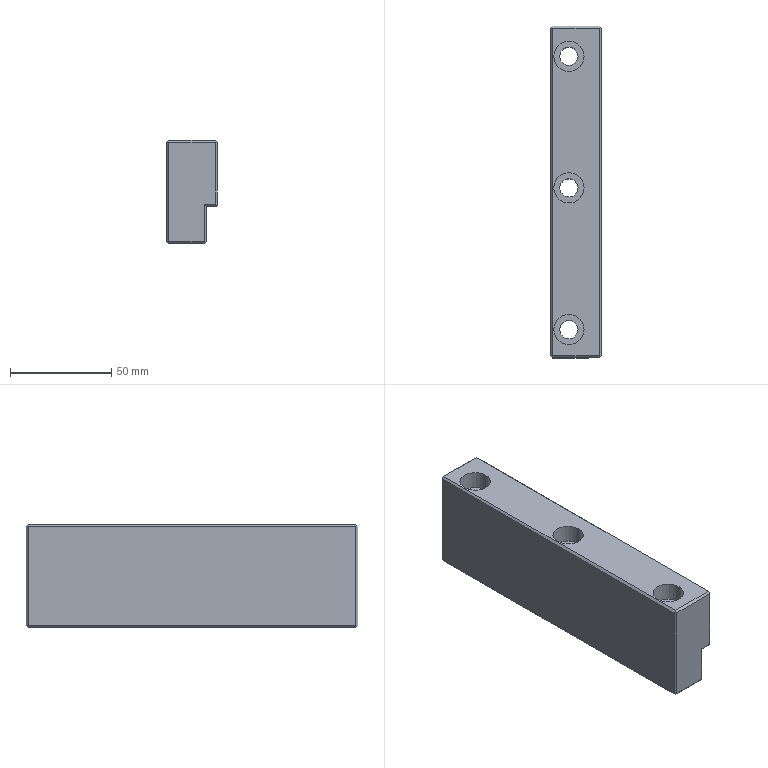Part | Creo | 1 solid | 39 faces | box 25 x 164 x 51 mm | volume 179141 mm3 | plane 27 | cylinder 12 | commonest cylinder face diameters 9 x6 15 x6
STEP:
#1=CARTESIAN_POINT('',(-98.742,211.92,-62.));
#2=VERTEX_POINT('',#1);
#3=CARTESIAN_POINT('',(-98.742,373.92,-62.));
#4=VERTEX_POINT('',#3);
#5=CARTESIAN_POINT('',(-98.742,211.92,-62.));
#6=DIRECTION('',(0.,1.,0.));
#7=VECTOR('',#6,162.);
#8=LINE('',#5,#7);
#9=EDGE_CURVE('',#2,#4,#8,.T.);
#10=ORIENTED_EDGE('',*,*,#9,.T.);
#11=CARTESIAN_POINT('',(-99.242,374.42,-61.5));
#12=VERTEX_POINT('',#11);
#13=CARTESIAN_POINT('',(-98.742,373.92,-62.));
#14=DIRECTION('',(-0.5774,0.5774,0.5774));
#15=VECTOR('',#14,0.866);
#16=LINE('',#13,#15);
#17=EDGE_CURVE('',#4,#12,#16,.T.);
#18=ORIENTED_EDGE('',*,*,#17,.T.);
#19=CARTESIAN_POINT('',(-99.742,373.92,-61.));
#20=VERTEX_POINT('',#19);
#21=CARTESIAN_POINT('',(-99.242,374.42,-61.5));
#22=DIRECTION('',(-0.5774,-0.5774,0.5774));
#23=VECTOR('',#22,0.866);
#24=LINE('',#21,#23);
#25=EDGE_CURVE('',#12,#20,#24,.T.);
#26=ORIENTED_EDGE('',*,*,#25,.T.);
#27=CARTESIAN_POINT('',(-99.742,211.92,-61.));
#28=VERTEX_POINT('',#27);
#29=CARTESIAN_POINT('',(-99.742,211.92,-61.));
#30=DIRECTION('',(0.,1.,0.));
#31=VECTOR('',#30,162.);
#32=LINE('',#29,#31);
#33=EDGE_CURVE('',#28,#20,#32,.T.);
#34=ORIENTED_EDGE('',*,*,#33,.F.);
#35=CARTESIAN_POINT('',(-99.242,211.42,-61.5));
#36=VERTEX_POINT('',#35);
#37=CARTESIAN_POINT('',(-99.742,211.92,-61.));
#38=DIRECTION('',(0.5774,-0.5774,-0.5774));
#39=VECTOR('',#38,0.866);
#40=LINE('',#37,#39);
#41=EDGE_CURVE('',#28,#36,#40,.T.);
#42=ORIENTED_EDGE('',*,*,#41,.T.);
#43=CARTESIAN_POINT('',(-98.742,211.92,-62.));
#44=DIRECTION('',(-0.5774,-0.5774,0.5774));
#45=VECTOR('',#44,0.866);
#46=LINE('',#43,#45);
#47=EDGE_CURVE('',#2,#36,#46,.T.);
#48=ORIENTED_EDGE('',*,*,#47,.F.);
#49=EDGE_LOOP('',(#10,#18,#26,#34,#42,#48));
#50=FACE_OUTER_BOUND('',#49,.F.);
#51=CARTESIAN_POINT('',(-99.242,279.92,-61.5));
#52=DIRECTION('',(-0.7071,0.,-0.7071));
#53=DIRECTION('',(-0.7071,0.,0.7071));
#54=AXIS2_PLACEMENT_3D('',#51,#52,#53);
#55=PLANE('',#54);
#56=ADVANCED_FACE('',(#50),#55,.T.);
#57=CARTESIAN_POINT('',(-81.242,211.92,-62.));
#58=VERTEX_POINT('',#57);
#59=CARTESIAN_POINT('',(-81.242,211.92,-62.));
#60=DIRECTION('',(-1.,0.,0.));
#61=VECTOR('',#60,17.5);
#62=LINE('',#59,#61);
#63=EDGE_CURVE('',#58,#2,#62,.T.);
#64=ORIENTED_EDGE('',*,*,#63,.F.);
#65=CARTESIAN_POINT('',(-81.242,373.92,-62.));
#66=VERTEX_POINT('',#65);
#67=CARTESIAN_POINT('',(-81.242,211.92,-62.));
#68=DIRECTION('',(0.,1.,0.));
#69=VECTOR('',#68,162.);
#70=LINE('',#67,#69);
#71=EDGE_CURVE('',#58,#66,#70,.T.);
#72=ORIENTED_EDGE('',*,*,#71,.T.);
#73=CARTESIAN_POINT('',(-98.742,373.92,-62.));
#74=DIRECTION('',(1.,0.,0.));
#75=VECTOR('',#74,17.5);
#76=LINE('',#73,#75);
#77=EDGE_CURVE('',#4,#66,#76,.T.);
#78=ORIENTED_EDGE('',*,*,#77,.F.);
#79=ORIENTED_EDGE('',*,*,#9,.F.);
#80=EDGE_LOOP('',(#64,#72,#78,#79));
#81=FACE_OUTER_BOUND('',#80,.F.);
#82=CARTESIAN_POINT('',(-86.242,359.92,-62.));
#83=VERTEX_POINT('',#82);
#84=CARTESIAN_POINT('',(-95.242,359.92,-62.));
#85=VERTEX_POINT('',#84);
#86=CARTESIAN_POINT('',(-90.742,359.92,-62.));
#87=DIRECTION('',(0.,0.,1.));
#88=DIRECTION('',(1.,0.,0.));
#89=AXIS2_PLACEMENT_3D('',#86,#87,#88);
#90=CIRCLE('',#89,4.5);
#91=EDGE_CURVE('',#83,#85,#90,.T.);
#92=ORIENTED_EDGE('',*,*,#91,.F.);
#93=CARTESIAN_POINT('',(-90.742,359.92,-62.));
#94=DIRECTION('',(0.,0.,1.));
#95=DIRECTION('',(-1.,0.,0.));
#96=AXIS2_PLACEMENT_3D('',#93,#94,#95);
#97=CIRCLE('',#96,4.5);
#98=EDGE_CURVE('',#85,#83,#97,.T.);
#99=ORIENTED_EDGE('',*,*,#98,.F.);
#100=EDGE_LOOP('',(#92,#99));
#101=FACE_BOUND('',#100,.F.);
#102=CARTESIAN_POINT('',(-86.242,294.92,-62.));
#103=VERTEX_POINT('',#102);
#104=CARTESIAN_POINT('',(-95.242,294.92,-62.));
#105=VERTEX_POINT('',#104);
#106=CARTESIAN_POINT('',(-90.742,294.92,-62.));
#107=DIRECTION('',(0.,0.,1.));
#108=DIRECTION('',(1.,0.,0.));
#109=AXIS2_PLACEMENT_3D('',#106,#107,#108);
#110=CIRCLE('',#109,4.5);
#111=EDGE_CURVE('',#103,#105,#110,.T.);
#112=ORIENTED_EDGE('',*,*,#111,.F.);
#113=CARTESIAN_POINT('',(-90.742,294.92,-62.));
#114=DIRECTION('',(0.,0.,1.));
#115=DIRECTION('',(-1.,0.,0.));
#116=AXIS2_PLACEMENT_3D('',#113,#114,#115);
#117=CIRCLE('',#116,4.5);
#118=EDGE_CURVE('',#105,#103,#117,.T.);
#119=ORIENTED_EDGE('',*,*,#118,.F.);
#120=EDGE_LOOP('',(#112,#119));
#121=FACE_BOUND('',#120,.F.);
#122=CARTESIAN_POINT('',(-86.242,224.92,-62.));
#123=VERTEX_POINT('',#122);
#124=CARTESIAN_POINT('',(-95.242,224.92,-62.));
#125=VERTEX_POINT('',#124);
#126=CARTESIAN_POINT('',(-90.742,224.92,-62.));
#127=DIRECTION('',(0.,0.,1.));
#128=DIRECTION('',(1.,0.,0.));
#129=AXIS2_PLACEMENT_3D('',#126,#127,#128);
#130=CIRCLE('',#129,4.5);
#131=EDGE_CURVE('',#123,#125,#130,.T.);
#132=ORIENTED_EDGE('',*,*,#131,.F.);
#133=CARTESIAN_POINT('',(-90.742,224.92,-62.));
#134=DIRECTION('',(0.,0.,1.));
#135=DIRECTION('',(-1.,0.,0.));
#136=AXIS2_PLACEMENT_3D('',#133,#134,#135);
#137=CIRCLE('',#136,4.5);
#138=EDGE_CURVE('',#125,#123,#137,.T.);
#139=ORIENTED_EDGE('',*,*,#138,.F.);
#140=EDGE_LOOP('',(#132,#139));
#141=FACE_BOUND('',#140,.F.);
#142=CARTESIAN_POINT('',(-80.242,349.92,-62.));
#143=DIRECTION('',(0.,0.,-1.));
#144=DIRECTION('',(1.,0.,0.));
#145=AXIS2_PLACEMENT_3D('',#142,#143,#144);
#146=PLANE('',#145);
#147=ADVANCED_FACE('',(#81,#101,#121,#141),#146,.T.);
#148=ORIENTED_EDGE('',*,*,#63,.T.);
#149=ORIENTED_EDGE('',*,*,#47,.T.);
#150=CARTESIAN_POINT('',(-98.742,210.92,-61.));
#151=VERTEX_POINT('',#150);
#152=CARTESIAN_POINT('',(-99.242,211.42,-61.5));
#153=DIRECTION('',(0.5774,-0.5774,0.5774));
#154=VECTOR('',#153,0.866);
#155=LINE('',#152,#154);
#156=EDGE_CURVE('',#36,#151,#155,.T.);
#157=ORIENTED_EDGE('',*,*,#156,.T.);
#158=CARTESIAN_POINT('',(-81.242,210.92,-61.));
#159=VERTEX_POINT('',#158);
#160=CARTESIAN_POINT('',(-81.242,210.92,-61.));
#161=DIRECTION('',(-1.,0.,0.));
#162=VECTOR('',#161,17.5);
#163=LINE('',#160,#162);
#164=EDGE_CURVE('',#159,#151,#163,.T.);
#165=ORIENTED_EDGE('',*,*,#164,.F.);
#166=CARTESIAN_POINT('',(-80.742,211.42,-61.5));
#167=VERTEX_POINT('',#166);
#168=CARTESIAN_POINT('',(-81.242,210.92,-61.));
#169=DIRECTION('',(0.5774,0.5774,-0.5774));
#170=VECTOR('',#169,0.866);
#171=LINE('',#168,#170);
#172=EDGE_CURVE('',#159,#167,#171,.T.);
#173=ORIENTED_EDGE('',*,*,#172,.T.);
#174=CARTESIAN_POINT('',(-80.742,211.42,-61.5));
#175=DIRECTION('',(-0.5774,0.5774,-0.5774));
#176=VECTOR('',#175,0.866);
#177=LINE('',#174,#176);
#178=EDGE_CURVE('',#167,#58,#177,.T.);
#179=ORIENTED_EDGE('',*,*,#178,.T.);
#180=EDGE_LOOP('',(#148,#149,#157,#165,#173,#179));
#181=FACE_OUTER_BOUND('',#180,.F.);
#182=CARTESIAN_POINT('',(-89.992,211.42,-61.5));
#183=DIRECTION('',(0.,-0.7071,-0.7071));
#184=DIRECTION('',(0.,-0.7071,0.7071));
#185=AXIS2_PLACEMENT_3D('',#182,#183,#184);
#186=PLANE('',#185);
#187=ADVANCED_FACE('',(#181),#186,.T.);
#188=CARTESIAN_POINT('',(-98.742,210.92,-12.));
#189=VERTEX_POINT('',#188);
#190=CARTESIAN_POINT('',(-98.742,210.92,-61.));
#191=DIRECTION('',(0.,0.,1.));
#192=VECTOR('',#191,49.);
#193=LINE('',#190,#192);
#194=EDGE_CURVE('',#151,#189,#193,.T.);
#195=ORIENTED_EDGE('',*,*,#194,.F.);
#196=ORIENTED_EDGE('',*,*,#156,.F.);
#197=ORIENTED_EDGE('',*,*,#41,.F.);
#198=CARTESIAN_POINT('',(-99.742,211.92,-12.));
#199=VERTEX_POINT('',#198);
#200=CARTESIAN_POINT('',(-99.742,211.92,-61.));
#201=DIRECTION('',(0.,0.,1.));
#202=VECTOR('',#201,49.);
#203=LINE('',#200,#202);
#204=EDGE_CURVE('',#28,#199,#203,.T.);
#205=ORIENTED_EDGE('',*,*,#204,.T.);
#206=CARTESIAN_POINT('',(-99.242,211.42,-11.5));
#207=VERTEX_POINT('',#206);
#208=CARTESIAN_POINT('',(-99.242,211.42,-11.5));
#209=DIRECTION('',(-0.5774,0.5774,-0.5774));
#210=VECTOR('',#209,0.866);
#211=LINE('',#208,#210);
#212=EDGE_CURVE('',#207,#199,#211,.T.);
#213=ORIENTED_EDGE('',*,*,#212,.F.);
#214=CARTESIAN_POINT('',(-99.242,211.42,-11.5));
#215=DIRECTION('',(0.5774,-0.5774,-0.5774));
#216=VECTOR('',#215,0.866);
#217=LINE('',#214,#216);
#218=EDGE_CURVE('',#207,#189,#217,.T.);
#219=ORIENTED_EDGE('',*,*,#218,.T.);
#220=EDGE_LOOP('',(#195,#196,#197,#205,#213,#219));
#221=FACE_OUTER_BOUND('',#220,.F.);
#222=CARTESIAN_POINT('',(-99.242,211.42,-29.));
#223=DIRECTION('',(-0.7071,-0.7071,0.));
#224=DIRECTION('',(0.7071,-0.7071,0.));
#225=AXIS2_PLACEMENT_3D('',#222,#223,#224);
#226=PLANE('',#225);
#227=ADVANCED_FACE('',(#221),#226,.T.);
#228=CARTESIAN_POINT('',(-81.242,210.92,-42.5));
#229=VERTEX_POINT('',#228);
#230=CARTESIAN_POINT('',(-81.242,210.92,-42.5));
#231=DIRECTION('',(0.,0.,-1.));
#232=VECTOR('',#231,18.5);
#233=LINE('',#230,#232);
#234=EDGE_CURVE('',#229,#159,#233,.T.);
#235=ORIENTED_EDGE('',*,*,#234,.T.);
#236=ORIENTED_EDGE('',*,*,#164,.T.);
#237=ORIENTED_EDGE('',*,*,#194,.T.);
#238=CARTESIAN_POINT('',(-75.742,210.92,-12.));
#239=VERTEX_POINT('',#238);
#240=CARTESIAN_POINT('',(-98.742,210.92,-12.));
#241=DIRECTION('',(1.,0.,0.));
#242=VECTOR('',#241,23.);
#243=LINE('',#240,#242);
#244=EDGE_CURVE('',#189,#239,#243,.T.);
#245=ORIENTED_EDGE('',*,*,#244,.T.);
#246=CARTESIAN_POINT('',(-75.742,210.92,-42.5));
#247=VERTEX_POINT('',#246);
#248=CARTESIAN_POINT('',(-75.742,210.92,-12.));
#249=DIRECTION('',(0.,0.,-1.));
#250=VECTOR('',#249,30.5);
#251=LINE('',#248,#250);
#252=EDGE_CURVE('',#239,#247,#251,.T.);
#253=ORIENTED_EDGE('',*,*,#252,.T.);
#254=CARTESIAN_POINT('',(-75.742,210.92,-42.5));
#255=DIRECTION('',(-1.,0.,0.));
#256=VECTOR('',#255,5.5);
#257=LINE('',#254,#256);
#258=EDGE_CURVE('',#247,#229,#257,.T.);
#259=ORIENTED_EDGE('',*,*,#258,.T.);
#260=EDGE_LOOP('',(#235,#236,#237,#245,#253,#259));
#261=FACE_OUTER_BOUND('',#260,.F.);
#262=CARTESIAN_POINT('',(-80.242,210.92,-41.));
#263=DIRECTION('',(0.,-1.,0.));
#264=DIRECTION('',(0.,0.,-1.));
#265=AXIS2_PLACEMENT_3D('',#262,#263,#264);
#266=PLANE('',#265);
#267=ADVANCED_FACE('',(#261),#266,.T.);
#268=ORIENTED_EDGE('',*,*,#172,.F.);
#269=ORIENTED_EDGE('',*,*,#234,.F.);
#270=CARTESIAN_POINT('',(-80.242,211.92,-43.5));
#271=VERTEX_POINT('',#270);
#272=CARTESIAN_POINT('',(-80.242,211.92,-43.5));
#273=DIRECTION('',(-0.5774,-0.5774,0.5774));
#274=VECTOR('',#273,1.732);
#275=LINE('',#272,#274);
#276=EDGE_CURVE('',#271,#229,#275,.T.);
#277=ORIENTED_EDGE('',*,*,#276,.F.);
#278=CARTESIAN_POINT('',(-80.242,211.92,-61.));
#279=VERTEX_POINT('',#278);
#280=CARTESIAN_POINT('',(-80.242,211.92,-61.));
#281=DIRECTION('',(0.,0.,1.));
#282=VECTOR('',#281,17.5);
#283=LINE('',#280,#282);
#284=EDGE_CURVE('',#279,#271,#283,.T.);
#285=ORIENTED_EDGE('',*,*,#284,.F.);
#286=CARTESIAN_POINT('',(-80.242,211.92,-61.));
#287=DIRECTION('',(-0.5774,-0.5774,-0.5774));
#288=VECTOR('',#287,0.866);
#289=LINE('',#286,#288);
#290=EDGE_CURVE('',#279,#167,#289,.T.);
#291=ORIENTED_EDGE('',*,*,#290,.T.);
#292=EDGE_LOOP('',(#268,#269,#277,#285,#291));
#293=FACE_OUTER_BOUND('',#292,.F.);
#294=CARTESIAN_POINT('',(-80.742,211.42,-51.5));
#295=DIRECTION('',(0.7071,-0.7071,0.));
#296=DIRECTION('',(-0.7071,-0.7071,0.));
#297=AXIS2_PLACEMENT_3D('',#294,#295,#296);
#298=PLANE('',#297);
#299=ADVANCED_FACE('',(#293),#298,.T.);
#300=CARTESIAN_POINT('',(-75.242,211.92,-43.5));
#301=VERTEX_POINT('',#300);
#302=CARTESIAN_POINT('',(-75.242,211.92,-43.5));
#303=DIRECTION('',(-1.,0.,0.));
#304=VECTOR('',#303,5.);
#305=LINE('',#302,#304);
#306=EDGE_CURVE('',#301,#271,#305,.T.);
#307=ORIENTED_EDGE('',*,*,#306,.T.);
#308=ORIENTED_EDGE('',*,*,#276,.T.);
#309=ORIENTED_EDGE('',*,*,#258,.F.);
#310=CARTESIAN_POINT('',(-74.992,211.67,-43.25));
#311=VERTEX_POINT('',#310);
#312=CARTESIAN_POINT('',(-75.742,210.92,-42.5));
#313=DIRECTION('',(0.5774,0.5774,-0.5774));
#314=VECTOR('',#313,1.299);
#315=LINE('',#312,#314);
#316=EDGE_CURVE('',#247,#311,#315,.T.);
#317=ORIENTED_EDGE('',*,*,#316,.T.);
#318=CARTESIAN_POINT('',(-74.992,211.67,-43.25));
#319=DIRECTION('',(-0.5774,0.5774,-0.5774));
#320=VECTOR('',#319,0.433);
#321=LINE('',#318,#320);
#322=EDGE_CURVE('',#311,#301,#321,.T.);
#323=ORIENTED_EDGE('',*,*,#322,.T.);
#324=EDGE_LOOP('',(#307,#308,#309,#317,#323));
#325=FACE_OUTER_BOUND('',#324,.F.);
#326=CARTESIAN_POINT('',(-77.492,211.42,-43.));
#327=DIRECTION('',(0.,-0.7071,-0.7071));
#328=DIRECTION('',(0.,-0.7071,0.7071));
#329=AXIS2_PLACEMENT_3D('',#326,#327,#328);
#330=PLANE('',#329);
#331=ADVANCED_FACE('',(#325),#330,.T.);
#332=CARTESIAN_POINT('',(-80.242,373.92,-43.5));
#333=VERTEX_POINT('',#332);
#334=CARTESIAN_POINT('',(-75.242,373.92,-43.5));
#335=VERTEX_POINT('',#334);
#336=CARTESIAN_POINT('',(-80.242,373.92,-43.5));
#337=DIRECTION('',(1.,0.,0.));
#338=VECTOR('',#337,5.);
#339=LINE('',#336,#338);
#340=EDGE_CURVE('',#333,#335,#339,.T.);
#341=ORIENTED_EDGE('',*,*,#340,.F.);
#342=CARTESIAN_POINT('',(-80.242,373.92,-43.5));
#343=DIRECTION('',(0.,-1.,0.));
#344=VECTOR('',#343,162.);
#345=LINE('',#342,#344);
#346=EDGE_CURVE('',#333,#271,#345,.T.);
#347=ORIENTED_EDGE('',*,*,#346,.T.);
#348=ORIENTED_EDGE('',*,*,#306,.F.);
#349=CARTESIAN_POINT('',(-75.242,211.92,-43.5));
#350=DIRECTION('',(0.,1.,0.));
#351=VECTOR('',#350,162.);
#352=LINE('',#349,#351);
#353=EDGE_CURVE('',#301,#335,#352,.T.);
#354=ORIENTED_EDGE('',*,*,#353,.T.);
#355=EDGE_LOOP('',(#341,#347,#348,#354));
#356=FACE_OUTER_BOUND('',#355,.F.);
#357=CARTESIAN_POINT('',(-74.742,349.92,-43.5));
#358=DIRECTION('',(0.,0.,-1.));
#359=DIRECTION('',(1.,0.,0.));
#360=AXIS2_PLACEMENT_3D('',#357,#358,#359);
#361=PLANE('',#360);
#362=ADVANCED_FACE('',(#356),#361,.T.);
#363=CARTESIAN_POINT('',(-74.992,374.17,-43.25));
#364=VERTEX_POINT('',#363);
#365=CARTESIAN_POINT('',(-75.742,374.92,-42.5));
#366=VERTEX_POINT('',#365);
#367=CARTESIAN_POINT('',(-74.992,374.17,-43.25));
#368=DIRECTION('',(-0.5774,0.5774,0.5774));
#369=VECTOR('',#368,1.299);
#370=LINE('',#367,#369);
#371=EDGE_CURVE('',#364,#366,#370,.T.);
#372=ORIENTED_EDGE('',*,*,#371,.T.);
#373=CARTESIAN_POINT('',(-80.242,374.92,-42.5));
#374=VERTEX_POINT('',#373);
#375=CARTESIAN_POINT('',(-80.242,374.92,-42.5));
#376=DIRECTION('',(1.,0.,0.));
#377=VECTOR('',#376,4.5);
#378=LINE('',#375,#377);
#379=EDGE_CURVE('',#374,#366,#378,.T.);
#380=ORIENTED_EDGE('',*,*,#379,.F.);
#381=CARTESIAN_POINT('',(-80.242,374.92,-42.5));
#382=DIRECTION('',(0.,-0.7071,-0.7071));
#383=VECTOR('',#382,1.414);
#384=LINE('',#381,#383);
#385=EDGE_CURVE('',#374,#333,#384,.T.);
#386=ORIENTED_EDGE('',*,*,#385,.T.);
#387=ORIENTED_EDGE('',*,*,#340,.T.);
#388=CARTESIAN_POINT('',(-75.242,373.92,-43.5));
#389=DIRECTION('',(0.5774,0.5774,0.5774));
#390=VECTOR('',#389,0.433);
#391=LINE('',#388,#390);
#392=EDGE_CURVE('',#335,#364,#391,.T.);
#393=ORIENTED_EDGE('',*,*,#392,.T.);
#394=EDGE_LOOP('',(#372,#380,#386,#387,#393));
#395=FACE_OUTER_BOUND('',#394,.F.);
#396=CARTESIAN_POINT('',(-77.492,374.42,-43.));
#397=DIRECTION('',(0.,0.7071,-0.7071));
#398=DIRECTION('',(0.,0.7071,0.7071));
#399=AXIS2_PLACEMENT_3D('',#396,#397,#398);
#400=PLANE('',#399);
#401=ADVANCED_FACE('',(#395),#400,.T.);
#402=CARTESIAN_POINT('',(-74.742,373.92,-43.));
#403=VERTEX_POINT('',#402);
#404=CARTESIAN_POINT('',(-74.742,373.92,-12.));
#405=VERTEX_POINT('',#404);
#406=CARTESIAN_POINT('',(-74.742,373.92,-43.));
#407=DIRECTION('',(0.,0.,1.));
#408=VECTOR('',#407,31.);
#409=LINE('',#406,#408);
#410=EDGE_CURVE('',#403,#405,#409,.T.);
#411=ORIENTED_EDGE('',*,*,#410,.T.);
#412=CARTESIAN_POINT('',(-75.242,374.42,-11.5));
#413=VERTEX_POINT('',#412);
#414=CARTESIAN_POINT('',(-74.742,373.92,-12.));
#415=DIRECTION('',(-0.5774,0.5774,0.5774));
#416=VECTOR('',#415,0.866);
#417=LINE('',#414,#416);
#418=EDGE_CURVE('',#405,#413,#417,.T.);
#419=ORIENTED_EDGE('',*,*,#418,.T.);
#420=CARTESIAN_POINT('',(-75.742,374.92,-12.));
#421=VERTEX_POINT('',#420);
#422=CARTESIAN_POINT('',(-75.242,374.42,-11.5));
#423=DIRECTION('',(-0.5774,0.5774,-0.5774));
#424=VECTOR('',#423,0.866);
#425=LINE('',#422,#424);
#426=EDGE_CURVE('',#413,#421,#425,.T.);
#427=ORIENTED_EDGE('',*,*,#426,.T.);
#428=CARTESIAN_POINT('',(-75.742,374.92,-42.5));
#429=DIRECTION('',(0.,0.,1.));
#430=VECTOR('',#429,30.5);
#431=LINE('',#428,#430);
#432=EDGE_CURVE('',#366,#421,#431,.T.);
#433=ORIENTED_EDGE('',*,*,#432,.F.);
#434=ORIENTED_EDGE('',*,*,#371,.F.);
#435=CARTESIAN_POINT('',(-74.992,374.17,-43.25));
#436=DIRECTION('',(0.5774,-0.5774,0.5774));
#437=VECTOR('',#436,0.433);
#438=LINE('',#435,#437);
#439=EDGE_CURVE('',#364,#403,#438,.T.);
#440=ORIENTED_EDGE('',*,*,#439,.T.);
#441=EDGE_LOOP('',(#411,#419,#427,#433,#434,#440));
#442=FACE_OUTER_BOUND('',#441,.F.);
#443=CARTESIAN_POINT('',(-75.242,374.42,-21.));
#444=DIRECTION('',(0.7071,0.7071,0.));
#445=DIRECTION('',(-0.7071,0.7071,0.));
#446=AXIS2_PLACEMENT_3D('',#443,#444,#445);
#447=PLANE('',#446);
#448=ADVANCED_FACE('',(#442),#447,.T.);
#449=CARTESIAN_POINT('',(-74.742,211.92,-12.));
#450=VERTEX_POINT('',#449);
#451=CARTESIAN_POINT('',(-74.742,211.92,-43.));
#452=VERTEX_POINT('',#451);
#453=CARTESIAN_POINT('',(-74.742,211.92,-12.));
#454=DIRECTION('',(0.,0.,-1.));
#455=VECTOR('',#454,31.);
#456=LINE('',#453,#455);
#457=EDGE_CURVE('',#450,#452,#456,.T.);
#458=ORIENTED_EDGE('',*,*,#457,.F.);
#459=CARTESIAN_POINT('',(-74.742,211.92,-12.));
#460=DIRECTION('',(0.,1.,0.));
#461=VECTOR('',#460,162.);
#462=LINE('',#459,#461);
#463=EDGE_CURVE('',#450,#405,#462,.T.);
#464=ORIENTED_EDGE('',*,*,#463,.T.);
#465=ORIENTED_EDGE('',*,*,#410,.F.);
#466=CARTESIAN_POINT('',(-74.742,211.92,-43.));
#467=DIRECTION('',(0.,1.,0.));
#468=VECTOR('',#467,162.);
#469=LINE('',#466,#468);
#470=EDGE_CURVE('',#452,#403,#469,.T.);
#471=ORIENTED_EDGE('',*,*,#470,.F.);
#472=EDGE_LOOP('',(#458,#464,#465,#471));
#473=FACE_OUTER_BOUND('',#472,.F.);
#474=CARTESIAN_POINT('',(-74.742,349.92,-1.));
#475=DIRECTION('',(1.,0.,0.));
#476=DIRECTION('',(0.,0.,1.));
#477=AXIS2_PLACEMENT_3D('',#474,#475,#476);
#478=PLANE('',#477);
#479=ADVANCED_FACE('',(#473),#478,.T.);
#480=CARTESIAN_POINT('',(-75.242,211.42,-11.5));
#481=VERTEX_POINT('',#480);
#482=CARTESIAN_POINT('',(-74.742,211.92,-12.));
#483=DIRECTION('',(-0.5774,-0.5774,0.5774));
#484=VECTOR('',#483,0.866);
#485=LINE('',#482,#484);
#486=EDGE_CURVE('',#450,#481,#485,.T.);
#487=ORIENTED_EDGE('',*,*,#486,.F.);
#488=ORIENTED_EDGE('',*,*,#457,.T.);
#489=CARTESIAN_POINT('',(-74.742,211.92,-43.));
#490=DIRECTION('',(-0.5774,-0.5774,-0.5774));
#491=VECTOR('',#490,0.433);
#492=LINE('',#489,#491);
#493=EDGE_CURVE('',#452,#311,#492,.T.);
#494=ORIENTED_EDGE('',*,*,#493,.T.);
#495=ORIENTED_EDGE('',*,*,#316,.F.);
#496=ORIENTED_EDGE('',*,*,#252,.F.);
#497=CARTESIAN_POINT('',(-75.742,210.92,-12.));
#498=DIRECTION('',(0.5774,0.5774,0.5774));
#499=VECTOR('',#498,0.866);
#500=LINE('',#497,#499);
#501=EDGE_CURVE('',#239,#481,#500,.T.);
#502=ORIENTED_EDGE('',*,*,#501,.T.);
#503=EDGE_LOOP('',(#487,#488,#494,#495,#496,#502));
#504=FACE_OUTER_BOUND('',#503,.F.);
#505=CARTESIAN_POINT('',(-75.242,211.42,-21.));
#506=DIRECTION('',(0.7071,-0.7071,0.));
#507=DIRECTION('',(-0.7071,-0.7071,0.));
#508=AXIS2_PLACEMENT_3D('',#505,#506,#507);
#509=PLANE('',#508);
#510=ADVANCED_FACE('',(#504),#509,.T.);
#511=CARTESIAN_POINT('',(-75.742,211.92,-11.));
#512=VERTEX_POINT('',#511);
#513=CARTESIAN_POINT('',(-75.742,373.92,-11.));
#514=VERTEX_POINT('',#513);
#515=CARTESIAN_POINT('',(-75.742,211.92,-11.));
#516=DIRECTION('',(0.,1.,0.));
#517=VECTOR('',#516,162.);
#518=LINE('',#515,#517);
#519=EDGE_CURVE('',#512,#514,#518,.T.);
#520=ORIENTED_EDGE('',*,*,#519,.T.);
#521=CARTESIAN_POINT('',(-75.742,373.92,-11.));
#522=DIRECTION('',(0.5774,0.5774,-0.5774));
#523=VECTOR('',#522,0.866);
#524=LINE('',#521,#523);
#525=EDGE_CURVE('',#514,#413,#524,.T.);
#526=ORIENTED_EDGE('',*,*,#525,.T.);
#527=ORIENTED_EDGE('',*,*,#418,.F.);
#528=ORIENTED_EDGE('',*,*,#463,.F.);
#529=ORIENTED_EDGE('',*,*,#486,.T.);
#530=CARTESIAN_POINT('',(-75.242,211.42,-11.5));
#531=DIRECTION('',(-0.5774,0.5774,0.5774));
#532=VECTOR('',#531,0.866);
#533=LINE('',#530,#532);
#534=EDGE_CURVE('',#481,#512,#533,.T.);
#535=ORIENTED_EDGE('',*,*,#534,.T.);
#536=EDGE_LOOP('',(#520,#526,#527,#528,#529,#535));
#537=FACE_OUTER_BOUND('',#536,.F.);
#538=CARTESIAN_POINT('',(-75.242,279.92,-11.5));
#539=DIRECTION('',(0.7071,0.,0.7071));
#540=DIRECTION('',(0.7071,0.,-0.7071));
#541=AXIS2_PLACEMENT_3D('',#538,#539,#540);
#542=PLANE('',#541);
#543=ADVANCED_FACE('',(#537),#542,.T.);
#544=CARTESIAN_POINT('',(-98.742,211.92,-11.));
#545=VERTEX_POINT('',#544);
#546=CARTESIAN_POINT('',(-98.742,373.92,-11.));
#547=VERTEX_POINT('',#546);
#548=CARTESIAN_POINT('',(-98.742,211.92,-11.));
#549=DIRECTION('',(0.,1.,0.));
#550=VECTOR('',#549,162.);
#551=LINE('',#548,#550);
#552=EDGE_CURVE('',#545,#547,#551,.T.);
#553=ORIENTED_EDGE('',*,*,#552,.T.);
#554=CARTESIAN_POINT('',(-75.742,373.92,-11.));
#555=DIRECTION('',(-1.,0.,0.));
#556=VECTOR('',#555,23.);
#557=LINE('',#554,#556);
#558=EDGE_CURVE('',#514,#547,#557,.T.);
#559=ORIENTED_EDGE('',*,*,#558,.F.);
#560=ORIENTED_EDGE('',*,*,#519,.F.);
#561=CARTESIAN_POINT('',(-98.742,211.92,-11.));
#562=DIRECTION('',(1.,0.,0.));
#563=VECTOR('',#562,23.);
#564=LINE('',#561,#563);
#565=EDGE_CURVE('',#545,#512,#564,.T.);
#566=ORIENTED_EDGE('',*,*,#565,.F.);
#567=EDGE_LOOP('',(#553,#559,#560,#566));
#568=FACE_OUTER_BOUND('',#567,.F.);
#569=CARTESIAN_POINT('',(-83.242,294.92,-11.));
#570=VERTEX_POINT('',#569);
#571=CARTESIAN_POINT('',(-98.242,294.92,-11.));
#572=VERTEX_POINT('',#571);
#573=CARTESIAN_POINT('',(-90.742,294.92,-11.));
#574=DIRECTION('',(0.,0.,-1.));
#575=DIRECTION('',(1.,0.,0.));
#576=AXIS2_PLACEMENT_3D('',#573,#574,#575);
#577=CIRCLE('',#576,7.5);
#578=EDGE_CURVE('',#570,#572,#577,.T.);
#579=ORIENTED_EDGE('',*,*,#578,.F.);
#580=CARTESIAN_POINT('',(-90.742,294.92,-11.));
#581=DIRECTION('',(0.,0.,-1.));
#582=DIRECTION('',(-1.,0.,0.));
#583=AXIS2_PLACEMENT_3D('',#580,#581,#582);
#584=CIRCLE('',#583,7.5);
#585=EDGE_CURVE('',#572,#570,#584,.T.);
#586=ORIENTED_EDGE('',*,*,#585,.F.);
#587=EDGE_LOOP('',(#579,#586));
#588=FACE_BOUND('',#587,.F.);
#589=CARTESIAN_POINT('',(-83.242,359.92,-11.));
#590=VERTEX_POINT('',#589);
#591=CARTESIAN_POINT('',(-98.242,359.92,-11.));
#592=VERTEX_POINT('',#591);
#593=CARTESIAN_POINT('',(-90.742,359.92,-11.));
#594=DIRECTION('',(0.,0.,-1.));
#595=DIRECTION('',(1.,0.,0.));
#596=AXIS2_PLACEMENT_3D('',#593,#594,#595);
#597=CIRCLE('',#596,7.5);
#598=EDGE_CURVE('',#590,#592,#597,.T.);
#599=ORIENTED_EDGE('',*,*,#598,.F.);
#600=CARTESIAN_POINT('',(-90.742,359.92,-11.));
#601=DIRECTION('',(0.,0.,-1.));
#602=DIRECTION('',(-1.,0.,0.));
#603=AXIS2_PLACEMENT_3D('',#600,#601,#602);
#604=CIRCLE('',#603,7.5);
#605=EDGE_CURVE('',#592,#590,#604,.T.);
#606=ORIENTED_EDGE('',*,*,#605,.F.);
#607=EDGE_LOOP('',(#599,#606));
#608=FACE_BOUND('',#607,.F.);
#609=CARTESIAN_POINT('',(-83.242,224.92,-11.));
#610=VERTEX_POINT('',#609);
#611=CARTESIAN_POINT('',(-98.242,224.92,-11.));
#612=VERTEX_POINT('',#611);
#613=CARTESIAN_POINT('',(-90.742,224.92,-11.));
#614=DIRECTION('',(0.,0.,-1.));
#615=DIRECTION('',(1.,0.,0.));
#616=AXIS2_PLACEMENT_3D('',#613,#614,#615);
#617=CIRCLE('',#616,7.5);
#618=EDGE_CURVE('',#610,#612,#617,.T.);
#619=ORIENTED_EDGE('',*,*,#618,.F.);
#620=CARTESIAN_POINT('',(-90.742,224.92,-11.));
#621=DIRECTION('',(0.,0.,-1.));
#622=DIRECTION('',(-1.,0.,0.));
#623=AXIS2_PLACEMENT_3D('',#620,#621,#622);
#624=CIRCLE('',#623,7.5);
#625=EDGE_CURVE('',#612,#610,#624,.T.);
#626=ORIENTED_EDGE('',*,*,#625,.F.);
#627=EDGE_LOOP('',(#619,#626));
#628=FACE_BOUND('',#627,.F.);
#629=CARTESIAN_POINT('',(-99.742,349.92,-11.));
#630=DIRECTION('',(0.,0.,1.));
#631=DIRECTION('',(-1.,0.,0.));
#632=AXIS2_PLACEMENT_3D('',#629,#630,#631);
#633=PLANE('',#632);
#634=ADVANCED_FACE('',(#568,#588,#608,#628),#633,.T.);
#635=CARTESIAN_POINT('',(-98.742,211.92,-11.));
#636=DIRECTION('',(-0.5774,-0.5774,-0.5774));
#637=VECTOR('',#636,0.866);
#638=LINE('',#635,#637);
#639=EDGE_CURVE('',#545,#207,#638,.T.);
#640=ORIENTED_EDGE('',*,*,#639,.T.);
#641=ORIENTED_EDGE('',*,*,#212,.T.);
#642=CARTESIAN_POINT('',(-99.742,373.92,-12.));
#643=VERTEX_POINT('',#642);
#644=CARTESIAN_POINT('',(-99.742,211.92,-12.));
#645=DIRECTION('',(0.,1.,0.));
#646=VECTOR('',#645,162.);
#647=LINE('',#644,#646);
#648=EDGE_CURVE('',#199,#643,#647,.T.);
#649=ORIENTED_EDGE('',*,*,#648,.T.);
#650=CARTESIAN_POINT('',(-99.242,374.42,-11.5));
#651=VERTEX_POINT('',#650);
#652=CARTESIAN_POINT('',(-99.742,373.92,-12.));
#653=DIRECTION('',(0.5774,0.5774,0.5774));
#654=VECTOR('',#653,0.866);
#655=LINE('',#652,#654);
#656=EDGE_CURVE('',#643,#651,#655,.T.);
#657=ORIENTED_EDGE('',*,*,#656,.T.);
#658=CARTESIAN_POINT('',(-98.742,373.92,-11.));
#659=DIRECTION('',(-0.5774,0.5774,-0.5774));
#660=VECTOR('',#659,0.866);
#661=LINE('',#658,#660);
#662=EDGE_CURVE('',#547,#651,#661,.T.);
#663=ORIENTED_EDGE('',*,*,#662,.F.);
#664=ORIENTED_EDGE('',*,*,#552,.F.);
#665=EDGE_LOOP('',(#640,#641,#649,#657,#663,#664));
#666=FACE_OUTER_BOUND('',#665,.F.);
#667=CARTESIAN_POINT('',(-99.242,279.92,-11.5));
#668=DIRECTION('',(-0.7071,0.,0.7071));
#669=DIRECTION('',(0.7071,0.,0.7071));
#670=AXIS2_PLACEMENT_3D('',#667,#668,#669);
#671=PLANE('',#670);
#672=ADVANCED_FACE('',(#666),#671,.T.);
#673=ORIENTED_EDGE('',*,*,#244,.F.);
#674=ORIENTED_EDGE('',*,*,#218,.F.);
#675=ORIENTED_EDGE('',*,*,#639,.F.);
#676=ORIENTED_EDGE('',*,*,#565,.T.);
#677=ORIENTED_EDGE('',*,*,#534,.F.);
#678=ORIENTED_EDGE('',*,*,#501,.F.);
#679=EDGE_LOOP('',(#673,#674,#675,#676,#677,#678));
#680=FACE_OUTER_BOUND('',#679,.F.);
#681=CARTESIAN_POINT('',(-87.242,211.42,-11.5));
#682=DIRECTION('',(0.,-0.7071,0.7071));
#683=DIRECTION('',(0.,-0.7071,-0.7071));
#684=AXIS2_PLACEMENT_3D('',#681,#682,#683);
#685=PLANE('',#684);
#686=ADVANCED_FACE('',(#680),#685,.T.);
#687=ORIENTED_EDGE('',*,*,#204,.F.);
#688=ORIENTED_EDGE('',*,*,#33,.T.);
#689=CARTESIAN_POINT('',(-99.742,373.92,-12.));
#690=DIRECTION('',(0.,0.,-1.));
#691=VECTOR('',#690,49.);
#692=LINE('',#689,#691);
#693=EDGE_CURVE('',#643,#20,#692,.T.);
#694=ORIENTED_EDGE('',*,*,#693,.F.);
#695=ORIENTED_EDGE('',*,*,#648,.F.);
#696=EDGE_LOOP('',(#687,#688,#694,#695));
#697=FACE_OUTER_BOUND('',#696,.F.);
#698=CARTESIAN_POINT('',(-99.742,349.92,-57.));
#699=DIRECTION('',(-1.,0.,0.));
#700=DIRECTION('',(0.,0.,-1.));
#701=AXIS2_PLACEMENT_3D('',#698,#699,#700);
#702=PLANE('',#701);
#703=ADVANCED_FACE('',(#697),#702,.T.);
#704=ORIENTED_EDGE('',*,*,#25,.F.);
#705=CARTESIAN_POINT('',(-98.742,374.92,-61.));
#706=VERTEX_POINT('',#705);
#707=CARTESIAN_POINT('',(-98.742,374.92,-61.));
#708=DIRECTION('',(-0.5774,-0.5774,-0.5774));
#709=VECTOR('',#708,0.866);
#710=LINE('',#707,#709);
#711=EDGE_CURVE('',#706,#12,#710,.T.);
#712=ORIENTED_EDGE('',*,*,#711,.F.);
#713=CARTESIAN_POINT('',(-98.742,374.92,-12.));
#714=VERTEX_POINT('',#713);
#715=CARTESIAN_POINT('',(-98.742,374.92,-12.));
#716=DIRECTION('',(0.,0.,-1.));
#717=VECTOR('',#716,49.);
#718=LINE('',#715,#717);
#719=EDGE_CURVE('',#714,#706,#718,.T.);
#720=ORIENTED_EDGE('',*,*,#719,.F.);
#721=CARTESIAN_POINT('',(-99.242,374.42,-11.5));
#722=DIRECTION('',(0.5774,0.5774,-0.5774));
#723=VECTOR('',#722,0.866);
#724=LINE('',#721,#723);
#725=EDGE_CURVE('',#651,#714,#724,.T.);
#726=ORIENTED_EDGE('',*,*,#725,.F.);
#727=ORIENTED_EDGE('',*,*,#656,.F.);
#728=ORIENTED_EDGE('',*,*,#693,.T.);
#729=EDGE_LOOP('',(#704,#712,#720,#726,#727,#728));
#730=FACE_OUTER_BOUND('',#729,.F.);
#731=CARTESIAN_POINT('',(-99.242,374.42,-29.));
#732=DIRECTION('',(-0.7071,0.7071,0.));
#733=DIRECTION('',(0.7071,0.7071,0.));
#734=AXIS2_PLACEMENT_3D('',#731,#732,#733);
#735=PLANE('',#734);
#736=ADVANCED_FACE('',(#730),#735,.T.);
#737=CARTESIAN_POINT('',(-80.242,374.92,-61.));
#738=VERTEX_POINT('',#737);
#739=CARTESIAN_POINT('',(-98.742,374.92,-61.));
#740=DIRECTION('',(1.,0.,0.));
#741=VECTOR('',#740,18.5);
#742=LINE('',#739,#741);
#743=EDGE_CURVE('',#706,#738,#742,.T.);
#744=ORIENTED_EDGE('',*,*,#743,.F.);
#745=ORIENTED_EDGE('',*,*,#711,.T.);
#746=ORIENTED_EDGE('',*,*,#17,.F.);
#747=ORIENTED_EDGE('',*,*,#77,.T.);
#748=CARTESIAN_POINT('',(-81.242,373.92,-62.));
#749=DIRECTION('',(0.5774,0.5774,0.5774));
#750=VECTOR('',#749,1.732);
#751=LINE('',#748,#750);
#752=EDGE_CURVE('',#66,#738,#751,.T.);
#753=ORIENTED_EDGE('',*,*,#752,.T.);
#754=EDGE_LOOP('',(#744,#745,#746,#747,#753));
#755=FACE_OUTER_BOUND('',#754,.F.);
#756=CARTESIAN_POINT('',(-89.992,374.42,-61.5));
#757=DIRECTION('',(0.,0.7071,-0.7071));
#758=DIRECTION('',(0.,0.7071,0.7071));
#759=AXIS2_PLACEMENT_3D('',#756,#757,#758);
#760=PLANE('',#759);
#761=ADVANCED_FACE('',(#755),#760,.T.);
#762=ORIENTED_EDGE('',*,*,#743,.T.);
#763=CARTESIAN_POINT('',(-80.242,374.92,-61.));
#764=DIRECTION('',(0.,0.,1.));
#765=VECTOR('',#764,18.5);
#766=LINE('',#763,#765);
#767=EDGE_CURVE('',#738,#374,#766,.T.);
#768=ORIENTED_EDGE('',*,*,#767,.T.);
#769=ORIENTED_EDGE('',*,*,#379,.T.);
#770=ORIENTED_EDGE('',*,*,#432,.T.);
#771=CARTESIAN_POINT('',(-75.742,374.92,-12.));
#772=DIRECTION('',(-1.,0.,0.));
#773=VECTOR('',#772,23.);
#774=LINE('',#771,#773);
#775=EDGE_CURVE('',#421,#714,#774,.T.);
#776=ORIENTED_EDGE('',*,*,#775,.T.);
#777=ORIENTED_EDGE('',*,*,#719,.T.);
#778=EDGE_LOOP('',(#762,#768,#769,#770,#776,#777));
#779=FACE_OUTER_BOUND('',#778,.F.);
#780=CARTESIAN_POINT('',(-80.242,374.92,-41.));
#781=DIRECTION('',(0.,-1.,0.));
#782=DIRECTION('',(0.,0.,-1.));
#783=AXIS2_PLACEMENT_3D('',#780,#781,#782);
#784=PLANE('',#783);
#785=ADVANCED_FACE('',(#779),#784,.F.);
#786=ORIENTED_EDGE('',*,*,#284,.T.);
#787=ORIENTED_EDGE('',*,*,#346,.F.);
#788=ORIENTED_EDGE('',*,*,#385,.F.);
#789=ORIENTED_EDGE('',*,*,#767,.F.);
#790=CARTESIAN_POINT('',(-80.242,374.92,-61.));
#791=DIRECTION('',(0.,-1.,0.));
#792=VECTOR('',#791,163.);
#793=LINE('',#790,#792);
#794=EDGE_CURVE('',#738,#279,#793,.T.);
#795=ORIENTED_EDGE('',*,*,#794,.T.);
#796=EDGE_LOOP('',(#786,#787,#788,#789,#795));
#797=FACE_OUTER_BOUND('',#796,.F.);
#798=CARTESIAN_POINT('',(-80.242,349.92,-43.5));
#799=DIRECTION('',(1.,0.,0.));
#800=DIRECTION('',(0.,0.,1.));
#801=AXIS2_PLACEMENT_3D('',#798,#799,#800);
#802=PLANE('',#801);
#803=ADVANCED_FACE('',(#797),#802,.T.);
#804=ORIENTED_EDGE('',*,*,#752,.F.);
#805=ORIENTED_EDGE('',*,*,#71,.F.);
#806=ORIENTED_EDGE('',*,*,#178,.F.);
#807=ORIENTED_EDGE('',*,*,#290,.F.);
#808=ORIENTED_EDGE('',*,*,#794,.F.);
#809=EDGE_LOOP('',(#804,#805,#806,#807,#808));
#810=FACE_OUTER_BOUND('',#809,.F.);
#811=CARTESIAN_POINT('',(-81.242,349.92,-62.));
#812=DIRECTION('',(-0.7071,0.,0.7071));
#813=DIRECTION('',(0.,-1.,0.));
#814=AXIS2_PLACEMENT_3D('',#811,#812,#813);
#815=PLANE('',#814);
#816=ADVANCED_FACE('',(#810),#815,.F.);
#817=ORIENTED_EDGE('',*,*,#426,.F.);
#818=ORIENTED_EDGE('',*,*,#525,.F.);
#819=ORIENTED_EDGE('',*,*,#558,.T.);
#820=ORIENTED_EDGE('',*,*,#662,.T.);
#821=ORIENTED_EDGE('',*,*,#725,.T.);
#822=ORIENTED_EDGE('',*,*,#775,.F.);
#823=EDGE_LOOP('',(#817,#818,#819,#820,#821,#822));
#824=FACE_OUTER_BOUND('',#823,.F.);
#825=CARTESIAN_POINT('',(-87.242,374.42,-11.5));
#826=DIRECTION('',(0.,0.7071,0.7071));
#827=DIRECTION('',(0.,0.7071,-0.7071));
#828=AXIS2_PLACEMENT_3D('',#825,#826,#827);
#829=PLANE('',#828);
#830=ADVANCED_FACE('',(#824),#829,.T.);
#831=ORIENTED_EDGE('',*,*,#578,.T.);
#832=CARTESIAN_POINT('',(-98.242,294.92,-20.));
#833=VERTEX_POINT('',#832);
#834=CARTESIAN_POINT('',(-98.242,294.92,-11.));
#835=DIRECTION('',(0.,0.,-1.));
#836=VECTOR('',#835,9.);
#837=LINE('',#834,#836);
#838=EDGE_CURVE('',#572,#833,#837,.T.);
#839=ORIENTED_EDGE('',*,*,#838,.T.);
#840=CARTESIAN_POINT('',(-83.242,294.92,-20.));
#841=VERTEX_POINT('',#840);
#842=CARTESIAN_POINT('',(-90.742,294.92,-20.));
#843=DIRECTION('',(0.,0.,1.));
#844=DIRECTION('',(-1.,0.,0.));
#845=AXIS2_PLACEMENT_3D('',#842,#843,#844);
#846=CIRCLE('',#845,7.5);
#847=EDGE_CURVE('',#833,#841,#846,.T.);
#848=ORIENTED_EDGE('',*,*,#847,.T.);
#849=CARTESIAN_POINT('',(-83.242,294.92,-11.));
#850=DIRECTION('',(0.,0.,-1.));
#851=VECTOR('',#850,9.);
#852=LINE('',#849,#851);
#853=EDGE_CURVE('',#570,#841,#852,.T.);
#854=ORIENTED_EDGE('',*,*,#853,.F.);
#855=EDGE_LOOP('',(#831,#839,#848,#854));
#856=FACE_OUTER_BOUND('',#855,.F.);
#857=CARTESIAN_POINT('',(-90.742,294.92,-10.55));
#858=DIRECTION('',(0.,0.,-1.));
#859=DIRECTION('',(1.,0.,0.));
#860=AXIS2_PLACEMENT_3D('',#857,#858,#859);
#861=CYLINDRICAL_SURFACE('',#860,7.5);
#862=ADVANCED_FACE('',(#856),#861,.F.);
#863=ORIENTED_EDGE('',*,*,#585,.T.);
#864=ORIENTED_EDGE('',*,*,#853,.T.);
#865=CARTESIAN_POINT('',(-90.742,294.92,-20.));
#866=DIRECTION('',(0.,0.,1.));
#867=DIRECTION('',(1.,0.,0.));
#868=AXIS2_PLACEMENT_3D('',#865,#866,#867);
#869=CIRCLE('',#868,7.5);
#870=EDGE_CURVE('',#841,#833,#869,.T.);
#871=ORIENTED_EDGE('',*,*,#870,.T.);
#872=ORIENTED_EDGE('',*,*,#838,.F.);
#873=EDGE_LOOP('',(#863,#864,#871,#872));
#874=FACE_OUTER_BOUND('',#873,.F.);
#875=CARTESIAN_POINT('',(-90.742,294.92,-10.55));
#876=DIRECTION('',(0.,0.,-1.));
#877=DIRECTION('',(1.,0.,0.));
#878=AXIS2_PLACEMENT_3D('',#875,#876,#877);
#879=CYLINDRICAL_SURFACE('',#878,7.5);
#880=ADVANCED_FACE('',(#874),#879,.F.);
#881=ORIENTED_EDGE('',*,*,#847,.F.);
#882=ORIENTED_EDGE('',*,*,#870,.F.);
#883=EDGE_LOOP('',(#881,#882));
#884=FACE_OUTER_BOUND('',#883,.F.);
#885=CARTESIAN_POINT('',(-86.242,294.92,-20.));
#886=VERTEX_POINT('',#885);
#887=CARTESIAN_POINT('',(-95.242,294.92,-20.));
#888=VERTEX_POINT('',#887);
#889=CARTESIAN_POINT('',(-90.742,294.92,-20.));
#890=DIRECTION('',(0.,0.,-1.));
#891=DIRECTION('',(1.,0.,0.));
#892=AXIS2_PLACEMENT_3D('',#889,#890,#891);
#893=CIRCLE('',#892,4.5);
#894=EDGE_CURVE('',#886,#888,#893,.T.);
#895=ORIENTED_EDGE('',*,*,#894,.F.);
#896=CARTESIAN_POINT('',(-90.742,294.92,-20.));
#897=DIRECTION('',(0.,0.,-1.));
#898=DIRECTION('',(-1.,0.,0.));
#899=AXIS2_PLACEMENT_3D('',#896,#897,#898);
#900=CIRCLE('',#899,4.5);
#901=EDGE_CURVE('',#888,#886,#900,.T.);
#902=ORIENTED_EDGE('',*,*,#901,.F.);
#903=EDGE_LOOP('',(#895,#902));
#904=FACE_BOUND('',#903,.F.);
#905=CARTESIAN_POINT('',(-90.742,294.92,-20.));
#906=DIRECTION('',(0.,0.,-1.));
#907=DIRECTION('',(1.,0.,0.));
#908=AXIS2_PLACEMENT_3D('',#905,#906,#907);
#909=PLANE('',#908);
#910=ADVANCED_FACE('',(#884,#904),#909,.F.);
#911=ORIENTED_EDGE('',*,*,#118,.T.);
#912=CARTESIAN_POINT('',(-86.242,294.92,-62.));
#913=DIRECTION('',(0.,0.,1.));
#914=VECTOR('',#913,42.);
#915=LINE('',#912,#914);
#916=EDGE_CURVE('',#103,#886,#915,.T.);
#917=ORIENTED_EDGE('',*,*,#916,.T.);
#918=ORIENTED_EDGE('',*,*,#894,.T.);
#919=CARTESIAN_POINT('',(-95.242,294.92,-62.));
#920=DIRECTION('',(0.,0.,1.));
#921=VECTOR('',#920,42.);
#922=LINE('',#919,#921);
#923=EDGE_CURVE('',#105,#888,#922,.T.);
#924=ORIENTED_EDGE('',*,*,#923,.F.);
#925=EDGE_LOOP('',(#911,#917,#918,#924));
#926=FACE_OUTER_BOUND('',#925,.F.);
#927=CARTESIAN_POINT('',(-90.742,294.92,-10.));
#928=DIRECTION('',(0.,0.,1.));
#929=DIRECTION('',(1.,0.,0.));
#930=AXIS2_PLACEMENT_3D('',#927,#928,#929);
#931=CYLINDRICAL_SURFACE('',#930,4.5);
#932=ADVANCED_FACE('',(#926),#931,.F.);
#933=ORIENTED_EDGE('',*,*,#111,.T.);
#934=ORIENTED_EDGE('',*,*,#923,.T.);
#935=ORIENTED_EDGE('',*,*,#901,.T.);
#936=ORIENTED_EDGE('',*,*,#916,.F.);
#937=EDGE_LOOP('',(#933,#934,#935,#936));
#938=FACE_OUTER_BOUND('',#937,.F.);
#939=CARTESIAN_POINT('',(-90.742,294.92,-10.));
#940=DIRECTION('',(0.,0.,1.));
#941=DIRECTION('',(1.,0.,0.));
#942=AXIS2_PLACEMENT_3D('',#939,#940,#941);
#943=CYLINDRICAL_SURFACE('',#942,4.5);
#944=ADVANCED_FACE('',(#938),#943,.F.);
#945=ORIENTED_EDGE('',*,*,#598,.T.);
#946=CARTESIAN_POINT('',(-98.242,359.92,-20.));
#947=VERTEX_POINT('',#946);
#948=CARTESIAN_POINT('',(-98.242,359.92,-11.));
#949=DIRECTION('',(0.,0.,-1.));
#950=VECTOR('',#949,9.);
#951=LINE('',#948,#950);
#952=EDGE_CURVE('',#592,#947,#951,.T.);
#953=ORIENTED_EDGE('',*,*,#952,.T.);
#954=CARTESIAN_POINT('',(-83.242,359.92,-20.));
#955=VERTEX_POINT('',#954);
#956=CARTESIAN_POINT('',(-90.742,359.92,-20.));
#957=DIRECTION('',(0.,0.,1.));
#958=DIRECTION('',(-1.,0.,0.));
#959=AXIS2_PLACEMENT_3D('',#956,#957,#958);
#960=CIRCLE('',#959,7.5);
#961=EDGE_CURVE('',#947,#955,#960,.T.);
#962=ORIENTED_EDGE('',*,*,#961,.T.);
#963=CARTESIAN_POINT('',(-83.242,359.92,-11.));
#964=DIRECTION('',(0.,0.,-1.));
#965=VECTOR('',#964,9.);
#966=LINE('',#963,#965);
#967=EDGE_CURVE('',#590,#955,#966,.T.);
#968=ORIENTED_EDGE('',*,*,#967,.F.);
#969=EDGE_LOOP('',(#945,#953,#962,#968));
#970=FACE_OUTER_BOUND('',#969,.F.);
#971=CARTESIAN_POINT('',(-90.742,359.92,-10.55));
#972=DIRECTION('',(0.,0.,-1.));
#973=DIRECTION('',(1.,0.,0.));
#974=AXIS2_PLACEMENT_3D('',#971,#972,#973);
#975=CYLINDRICAL_SURFACE('',#974,7.5);
#976=ADVANCED_FACE('',(#970),#975,.F.);
#977=ORIENTED_EDGE('',*,*,#605,.T.);
#978=ORIENTED_EDGE('',*,*,#967,.T.);
#979=CARTESIAN_POINT('',(-90.742,359.92,-20.));
#980=DIRECTION('',(0.,0.,1.));
#981=DIRECTION('',(1.,0.,0.));
#982=AXIS2_PLACEMENT_3D('',#979,#980,#981);
#983=CIRCLE('',#982,7.5);
#984=EDGE_CURVE('',#955,#947,#983,.T.);
#985=ORIENTED_EDGE('',*,*,#984,.T.);
#986=ORIENTED_EDGE('',*,*,#952,.F.);
#987=EDGE_LOOP('',(#977,#978,#985,#986));
#988=FACE_OUTER_BOUND('',#987,.F.);
#989=CARTESIAN_POINT('',(-90.742,359.92,-10.55));
#990=DIRECTION('',(0.,0.,-1.));
#991=DIRECTION('',(1.,0.,0.));
#992=AXIS2_PLACEMENT_3D('',#989,#990,#991);
#993=CYLINDRICAL_SURFACE('',#992,7.5);
#994=ADVANCED_FACE('',(#988),#993,.F.);
#995=ORIENTED_EDGE('',*,*,#961,.F.);
#996=ORIENTED_EDGE('',*,*,#984,.F.);
#997=EDGE_LOOP('',(#995,#996));
#998=FACE_OUTER_BOUND('',#997,.F.);
#999=CARTESIAN_POINT('',(-86.242,359.92,-20.));
#1000=VERTEX_POINT('',#999);
#1001=CARTESIAN_POINT('',(-95.242,359.92,-20.));
#1002=VERTEX_POINT('',#1001);
#1003=CARTESIAN_POINT('',(-90.742,359.92,-20.));
#1004=DIRECTION('',(0.,0.,-1.));
#1005=DIRECTION('',(1.,0.,0.));
#1006=AXIS2_PLACEMENT_3D('',#1003,#1004,#1005);
#1007=CIRCLE('',#1006,4.5);
#1008=EDGE_CURVE('',#1000,#1002,#1007,.T.);
#1009=ORIENTED_EDGE('',*,*,#1008,.F.);
#1010=CARTESIAN_POINT('',(-90.742,359.92,-20.));
#1011=DIRECTION('',(0.,0.,-1.));
#1012=DIRECTION('',(-1.,0.,0.));
#1013=AXIS2_PLACEMENT_3D('',#1010,#1011,#1012);
#1014=CIRCLE('',#1013,4.5);
#1015=EDGE_CURVE('',#1002,#1000,#1014,.T.);
#1016=ORIENTED_EDGE('',*,*,#1015,.F.);
#1017=EDGE_LOOP('',(#1009,#1016));
#1018=FACE_BOUND('',#1017,.F.);
#1019=CARTESIAN_POINT('',(-90.742,359.92,-20.));
#1020=DIRECTION('',(0.,0.,-1.));
#1021=DIRECTION('',(1.,0.,0.));
#1022=AXIS2_PLACEMENT_3D('',#1019,#1020,#1021);
#1023=PLANE('',#1022);
#1024=ADVANCED_FACE('',(#998,#1018),#1023,.F.);
#1025=ORIENTED_EDGE('',*,*,#98,.T.);
#1026=CARTESIAN_POINT('',(-86.242,359.92,-62.));
#1027=DIRECTION('',(0.,0.,1.));
#1028=VECTOR('',#1027,42.);
#1029=LINE('',#1026,#1028);
#1030=EDGE_CURVE('',#83,#1000,#1029,.T.);
#1031=ORIENTED_EDGE('',*,*,#1030,.T.);
#1032=ORIENTED_EDGE('',*,*,#1008,.T.);
#1033=CARTESIAN_POINT('',(-95.242,359.92,-62.));
#1034=DIRECTION('',(0.,0.,1.));
#1035=VECTOR('',#1034,42.);
#1036=LINE('',#1033,#1035);
#1037=EDGE_CURVE('',#85,#1002,#1036,.T.);
#1038=ORIENTED_EDGE('',*,*,#1037,.F.);
#1039=EDGE_LOOP('',(#1025,#1031,#1032,#1038));
#1040=FACE_OUTER_BOUND('',#1039,.F.);
#1041=CARTESIAN_POINT('',(-90.742,359.92,-10.));
#1042=DIRECTION('',(0.,0.,1.));
#1043=DIRECTION('',(1.,0.,0.));
#1044=AXIS2_PLACEMENT_3D('',#1041,#1042,#1043);
#1045=CYLINDRICAL_SURFACE('',#1044,4.5);
#1046=ADVANCED_FACE('',(#1040),#1045,.F.);
#1047=ORIENTED_EDGE('',*,*,#91,.T.);
#1048=ORIENTED_EDGE('',*,*,#1037,.T.);
#1049=ORIENTED_EDGE('',*,*,#1015,.T.);
#1050=ORIENTED_EDGE('',*,*,#1030,.F.);
#1051=EDGE_LOOP('',(#1047,#1048,#1049,#1050));
#1052=FACE_OUTER_BOUND('',#1051,.F.);
#1053=CARTESIAN_POINT('',(-90.742,359.92,-10.));
#1054=DIRECTION('',(0.,0.,1.));
#1055=DIRECTION('',(1.,0.,0.));
#1056=AXIS2_PLACEMENT_3D('',#1053,#1054,#1055);
#1057=CYLINDRICAL_SURFACE('',#1056,4.5);
#1058=ADVANCED_FACE('',(#1052),#1057,.F.);
#1059=ORIENTED_EDGE('',*,*,#618,.T.);
#1060=CARTESIAN_POINT('',(-98.242,224.92,-20.));
#1061=VERTEX_POINT('',#1060);
#1062=CARTESIAN_POINT('',(-98.242,224.92,-11.));
#1063=DIRECTION('',(0.,0.,-1.));
#1064=VECTOR('',#1063,9.);
#1065=LINE('',#1062,#1064);
#1066=EDGE_CURVE('',#612,#1061,#1065,.T.);
#1067=ORIENTED_EDGE('',*,*,#1066,.T.);
#1068=CARTESIAN_POINT('',(-83.242,224.92,-20.));
#1069=VERTEX_POINT('',#1068);
#1070=CARTESIAN_POINT('',(-90.742,224.92,-20.));
#1071=DIRECTION('',(0.,0.,1.));
#1072=DIRECTION('',(-1.,0.,0.));
#1073=AXIS2_PLACEMENT_3D('',#1070,#1071,#1072);
#1074=CIRCLE('',#1073,7.5);
#1075=EDGE_CURVE('',#1061,#1069,#1074,.T.);
#1076=ORIENTED_EDGE('',*,*,#1075,.T.);
#1077=CARTESIAN_POINT('',(-83.242,224.92,-11.));
#1078=DIRECTION('',(0.,0.,-1.));
#1079=VECTOR('',#1078,9.);
#1080=LINE('',#1077,#1079);
#1081=EDGE_CURVE('',#610,#1069,#1080,.T.);
#1082=ORIENTED_EDGE('',*,*,#1081,.F.);
#1083=EDGE_LOOP('',(#1059,#1067,#1076,#1082));
#1084=FACE_OUTER_BOUND('',#1083,.F.);
#1085=CARTESIAN_POINT('',(-90.742,224.92,-10.55));
#1086=DIRECTION('',(0.,0.,-1.));
#1087=DIRECTION('',(1.,0.,0.));
#1088=AXIS2_PLACEMENT_3D('',#1085,#1086,#1087);
#1089=CYLINDRICAL_SURFACE('',#1088,7.5);
#1090=ADVANCED_FACE('',(#1084),#1089,.F.);
#1091=ORIENTED_EDGE('',*,*,#625,.T.);
#1092=ORIENTED_EDGE('',*,*,#1081,.T.);
#1093=CARTESIAN_POINT('',(-90.742,224.92,-20.));
#1094=DIRECTION('',(0.,0.,1.));
#1095=DIRECTION('',(1.,0.,0.));
#1096=AXIS2_PLACEMENT_3D('',#1093,#1094,#1095);
#1097=CIRCLE('',#1096,7.5);
#1098=EDGE_CURVE('',#1069,#1061,#1097,.T.);
#1099=ORIENTED_EDGE('',*,*,#1098,.T.);
#1100=ORIENTED_EDGE('',*,*,#1066,.F.);
#1101=EDGE_LOOP('',(#1091,#1092,#1099,#1100));
#1102=FACE_OUTER_BOUND('',#1101,.F.);
#1103=CARTESIAN_POINT('',(-90.742,224.92,-10.55));
#1104=DIRECTION('',(0.,0.,-1.));
#1105=DIRECTION('',(1.,0.,0.));
#1106=AXIS2_PLACEMENT_3D('',#1103,#1104,#1105);
#1107=CYLINDRICAL_SURFACE('',#1106,7.5);
#1108=ADVANCED_FACE('',(#1102),#1107,.F.);
#1109=ORIENTED_EDGE('',*,*,#1075,.F.);
#1110=ORIENTED_EDGE('',*,*,#1098,.F.);
#1111=EDGE_LOOP('',(#1109,#1110));
#1112=FACE_OUTER_BOUND('',#1111,.F.);
#1113=CARTESIAN_POINT('',(-86.242,224.92,-20.));
#1114=VERTEX_POINT('',#1113);
#1115=CARTESIAN_POINT('',(-95.242,224.92,-20.));
#1116=VERTEX_POINT('',#1115);
#1117=CARTESIAN_POINT('',(-90.742,224.92,-20.));
#1118=DIRECTION('',(0.,0.,-1.));
#1119=DIRECTION('',(1.,0.,0.));
#1120=AXIS2_PLACEMENT_3D('',#1117,#1118,#1119);
#1121=CIRCLE('',#1120,4.5);
#1122=EDGE_CURVE('',#1114,#1116,#1121,.T.);
#1123=ORIENTED_EDGE('',*,*,#1122,.F.);
#1124=CARTESIAN_POINT('',(-90.742,224.92,-20.));
#1125=DIRECTION('',(0.,0.,-1.));
#1126=DIRECTION('',(-1.,0.,0.));
#1127=AXIS2_PLACEMENT_3D('',#1124,#1125,#1126);
#1128=CIRCLE('',#1127,4.5);
#1129=EDGE_CURVE('',#1116,#1114,#1128,.T.);
#1130=ORIENTED_EDGE('',*,*,#1129,.F.);
#1131=EDGE_LOOP('',(#1123,#1130));
#1132=FACE_BOUND('',#1131,.F.);
#1133=CARTESIAN_POINT('',(-90.742,224.92,-20.));
#1134=DIRECTION('',(0.,0.,-1.));
#1135=DIRECTION('',(1.,0.,0.));
#1136=AXIS2_PLACEMENT_3D('',#1133,#1134,#1135);
#1137=PLANE('',#1136);
#1138=ADVANCED_FACE('',(#1112,#1132),#1137,.F.);
#1139=ORIENTED_EDGE('',*,*,#138,.T.);
#1140=CARTESIAN_POINT('',(-86.242,224.92,-62.));
#1141=DIRECTION('',(0.,0.,1.));
#1142=VECTOR('',#1141,42.);
#1143=LINE('',#1140,#1142);
#1144=EDGE_CURVE('',#123,#1114,#1143,.T.);
#1145=ORIENTED_EDGE('',*,*,#1144,.T.);
#1146=ORIENTED_EDGE('',*,*,#1122,.T.);
#1147=CARTESIAN_POINT('',(-95.242,224.92,-62.));
#1148=DIRECTION('',(0.,0.,1.));
#1149=VECTOR('',#1148,42.);
#1150=LINE('',#1147,#1149);
#1151=EDGE_CURVE('',#125,#1116,#1150,.T.);
#1152=ORIENTED_EDGE('',*,*,#1151,.F.);
#1153=EDGE_LOOP('',(#1139,#1145,#1146,#1152));
#1154=FACE_OUTER_BOUND('',#1153,.F.);
#1155=CARTESIAN_POINT('',(-90.742,224.92,-10.));
#1156=DIRECTION('',(0.,0.,1.));
#1157=DIRECTION('',(1.,0.,0.));
#1158=AXIS2_PLACEMENT_3D('',#1155,#1156,#1157);
#1159=CYLINDRICAL_SURFACE('',#1158,4.5);
#1160=ADVANCED_FACE('',(#1154),#1159,.F.);
#1161=ORIENTED_EDGE('',*,*,#131,.T.);
#1162=ORIENTED_EDGE('',*,*,#1151,.T.);
#1163=ORIENTED_EDGE('',*,*,#1129,.T.);
#1164=ORIENTED_EDGE('',*,*,#1144,.F.);
#1165=EDGE_LOOP('',(#1161,#1162,#1163,#1164));
#1166=FACE_OUTER_BOUND('',#1165,.F.);
#1167=CARTESIAN_POINT('',(-90.742,224.92,-10.));
#1168=DIRECTION('',(0.,0.,1.));
#1169=DIRECTION('',(1.,0.,0.));
#1170=AXIS2_PLACEMENT_3D('',#1167,#1168,#1169);
#1171=CYLINDRICAL_SURFACE('',#1170,4.5);
#1172=ADVANCED_FACE('',(#1166),#1171,.F.);
#1173=ORIENTED_EDGE('',*,*,#353,.F.);
#1174=ORIENTED_EDGE('',*,*,#322,.F.);
#1175=ORIENTED_EDGE('',*,*,#493,.F.);
#1176=ORIENTED_EDGE('',*,*,#470,.T.);
#1177=ORIENTED_EDGE('',*,*,#439,.F.);
#1178=ORIENTED_EDGE('',*,*,#392,.F.);
#1179=EDGE_LOOP('',(#1173,#1174,#1175,#1176,#1177,#1178));
#1180=FACE_OUTER_BOUND('',#1179,.F.);
#1181=CARTESIAN_POINT('',(-74.992,279.92,-43.25));
#1182=DIRECTION('',(0.7071,0.,-0.7071));
#1183=DIRECTION('',(-0.7071,0.,-0.7071));
#1184=AXIS2_PLACEMENT_3D('',#1181,#1182,#1183);
#1185=PLANE('',#1184);
#1186=ADVANCED_FACE('',(#1180),#1185,.T.);
#1187=CLOSED_SHELL('',(#56,#147,#187,#227,#267,#299,#331,#362,#401,#448,#479,#510,#543,#634,#672,#686,#703,#736,#761,#785,#803,#816,#830,#862,#880,#910,#932,#944,#976,#994,#1024,#1046,#1058,#1090,#1108,#1138,#1160,#1172,#1186));
#1188=MANIFOLD_SOLID_BREP('',#1187);
#1189=(LENGTH_UNIT()NAMED_UNIT(*)SI_UNIT(.MILLI.,.METRE.));
#1190=UNCERTAINTY_MEASURE_WITH_UNIT(LENGTH_MEASURE(0.01735),#1189,'','');
#1191=(NAMED_UNIT(*)PLANE_ANGLE_UNIT()SI_UNIT($,.RADIAN.));
#1192=PLANE_ANGLE_MEASURE_WITH_UNIT(PLANE_ANGLE_MEASURE(0.01745),#1191);
#1193=(CONVERSION_BASED_UNIT('DEGREE',#1192)NAMED_UNIT(*)PLANE_ANGLE_UNIT());
#1194=(NAMED_UNIT(*)SI_UNIT($,.STERADIAN.)SOLID_ANGLE_UNIT());
#1195=(GEOMETRIC_REPRESENTATION_CONTEXT(3)GLOBAL_UNCERTAINTY_ASSIGNED_CONTEXT((#1190))GLOBAL_UNIT_ASSIGNED_CONTEXT((#1189,#1193,#1194))REPRESENTATION_CONTEXT('',''));
#1196=ADVANCED_BREP_SHAPE_REPRESENTATION('',(#1188),#1195);